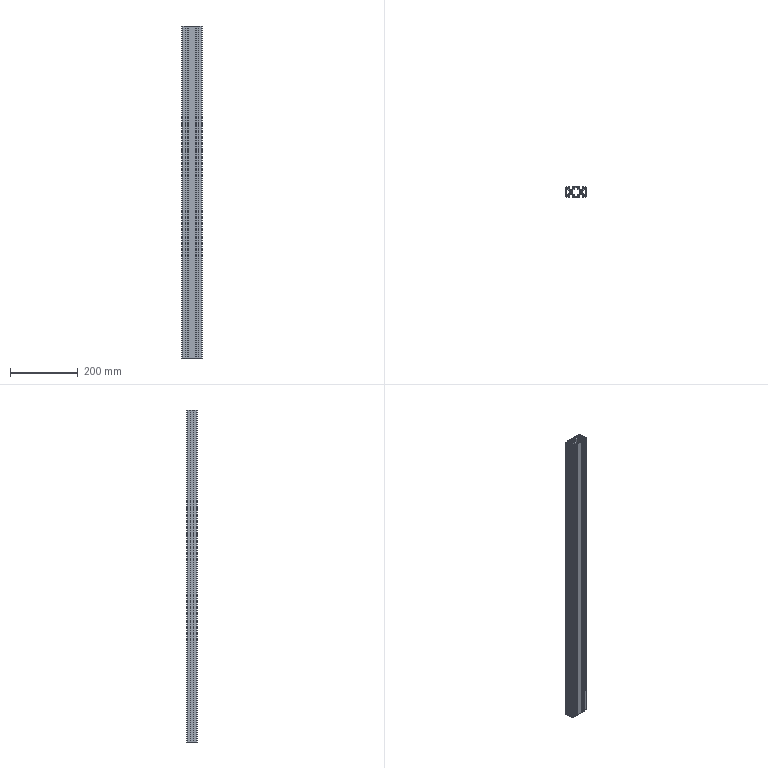Part | STEP file | SynoNew-0304-048 | 1 solid | 236 faces | box 60 x 30 x 980 mm | volume 587031 mm3 | cylinder 118 | plane 118 | commonest cylinder face diameters 0.6 x36 1.6 x36 4 x28 3 x8 6 x4 7 x4